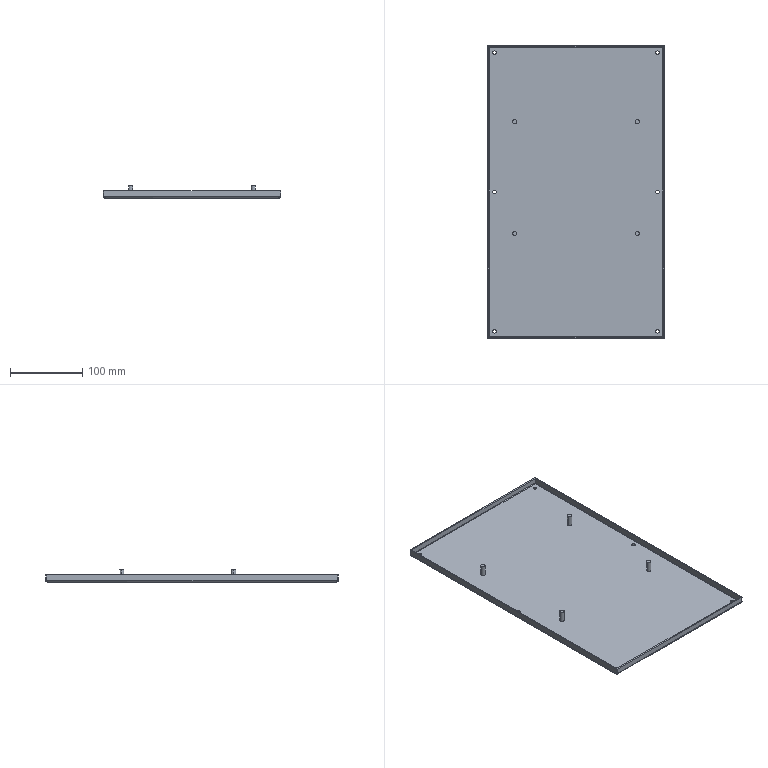Part | STEP file | Wrench controller box rear cover | 1 solid | 67 faces | box 246 x 406 x 17 mm | volume 220004 mm3 | cylinder 32 | spline 20 | plane 15 | commonest cylinder face diameters 5 x12 6 x8 1.473 x4 2 x4 5.473 x4